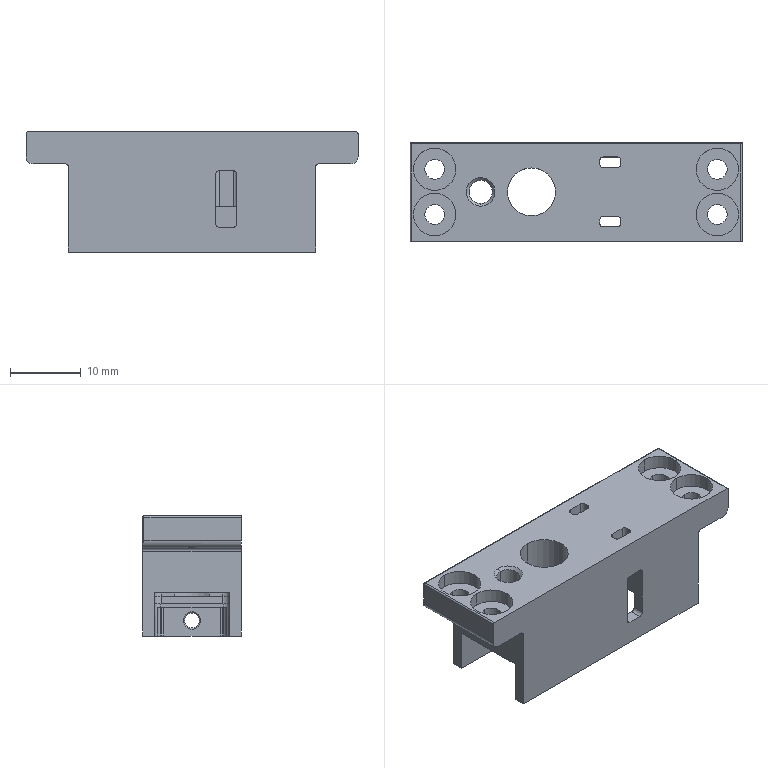NC program | NX | posted with a generic post | part box 47 x 14 x 17 mm
Lines 1055 to 1942 of 3166:
(CAVITY_MILL_COPY_COPY_COPY_COPY , TOOL : D1)
N2108 T22 M6
N2110 G54
N2112 G17 G0 G90 X-5.75 Y-1.208 B0. C0. S9200 M3
N2114 G43 Z30. H22
N2116 Z-0.065
N2118 G94 G3 X-5.85 Y-1.644 R1. F1000.
N2120 G1 Y-2.5 F850.
N2122 X-4.996
N2124 G3 X-4.696 Y-2.4 R0.5
N2126 G1 X-5.75 Y-1.208 Z-0.13 F8000.
N2128 G3 X-5.85 Y-1.644 R1. F1000.
N2130 G1 Y-2.5 F850.
N2132 X-4.996
N2134 G3 X-4.696 Y-2.4 R0.5
N2136 G1 X-5.75 Y-1.208 Z-0.195 F8000.
N2138 G3 X-5.85 Y-1.644 R1. F1000.
N2140 G1 Y-2.5 F850.
N2142 X-4.996
N2144 G3 X-4.696 Y-2.4 R0.5
N2146 G1 X-5.75 Y-1.208 Z-0.26 F8000.
N2148 G3 X-5.85 Y-1.644 R1. F1000.
N2150 G1 Y-2.5 F850.
N2152 X-4.996
N2154 G3 X-4.696 Y-2.4 R0.5
N2156 G1 X-5.75 Y-1.208 Z-0.325 F8000.
N2158 G3 X-5.85 Y-1.644 R1. F1000.
N2160 G1 Y-2.5 F850.
N2162 X-4.995
N2164 G3 X-4.695 Y-2.4 R0.5
N2166 G1 X-5.75 Y-1.208 Z-0.39 F8000.
N2168 G3 X-5.85 Y-1.644 R1. F1000.
N2170 G1 Y-2.5 F850.
N2172 X-4.995
N2174 G3 X-4.695 Y-2.4 R0.5
N2176 G1 X-5.75 Y-1.208 Z-0.455 F8000.
N2178 G3 X-5.85 Y-1.643 R1. F1000.
N2180 G1 Y-2.5 F850.
N2182 X-4.995
N2184 G3 X-4.695 Y-2.4 R0.5
N2186 G1 X-5.75 Y-1.207 Z-0.52 F8000.
N2188 G3 X-5.85 Y-1.643 R1. F1000.
N2190 G1 Y-2.5 F850.
N2192 X-4.995
N2194 G3 X-4.695 Y-2.4 R0.5
N2196 G1 X-5.75 Y-1.207 Z-0.585 F8000.
N2198 G3 X-5.85 Y-1.643 R1. F1000.
N2200 G1 Y-2.5 F850.
N2202 X-4.994
N2204 G3 X-4.694 Y-2.4 R0.5
N2206 G1 X-5.75 Y-1.207 Z-0.649 F8000.
N2208 G3 X-5.85 Y-1.643 R1. F1000.
N2210 G1 Y-2.5 F850.
N2212 X-4.994
N2214 G3 X-4.694 Y-2.4 R0.5
N2216 G1 X-5.75 Y-1.207 Z-0.714 F8000.
N2218 G3 X-5.85 Y-1.643 R1. F1000.
N2220 G1 Y-2.5 F850.
N2222 X-4.994
N2224 G3 X-4.694 Y-2.4 R0.5
N2226 G1 X-5.75 Y-1.207 Z-0.779 F8000.
N2228 G3 X-5.85 Y-1.643 R1. F1000.
N2230 G1 Y-2.5 F850.
N2232 X-4.994
N2234 G3 X-4.694 Y-2.4 R0.5
N2236 G1 X-5.75 Y-1.207 Z-0.844 F8000.
N2238 G3 X-5.85 Y-1.643 R1. F1000.
N2240 G1 Y-2.5 F850.
N2242 X-4.994
N2244 G3 X-4.694 Y-2.4 R0.5
N2246 G1 X-5.75 Y-1.207 Z-0.909 F8000.
N2248 G3 X-5.85 Y-1.643 R1. F1000.
N2250 G1 Y-2.5 F850.
N2252 X-4.993
N2254 G3 X-4.693 Y-2.4 R0.5
N2256 G1 X-5.75 Y-1.207 Z-0.974 F8000.
N2258 G3 X-5.85 Y-1.643 R1. F1000.
N2260 G1 Y-2.5 F850.
N2262 X-4.993
N2264 G3 X-4.693 Y-2.4 R0.5
N2266 G1 X-5.75 Y-1.207 Z-1.039 F8000.
N2268 G3 X-5.85 Y-1.643 R1. F1000.
N2270 G1 Y-2.5 F850.
N2272 X-4.993
N2274 G3 X-4.693 Y-2.4 R0.5
N2276 G1 X-5.75 Y-1.207 Z-1.104 F8000.
N2278 G3 X-5.85 Y-1.643 R1. F1000.
N2280 G1 Y-2.5 F850.
N2282 X-4.993
N2284 G3 X-4.693 Y-2.4 R0.5
N2286 G1 X-5.75 Y-1.207 Z-1.169 F8000.
N2288 G3 X-5.85 Y-1.643 R1. F1000.
N2290 G1 Y-2.5 F850.
N2292 X-4.992
N2294 G3 X-4.692 Y-2.4 R0.5
N2296 G1 X-5.75 Y-1.207 Z-1.234 F8000.
N2298 G3 X-5.85 Y-1.643 R1. F1000.
N2300 G1 Y-2.5 F850.
N2302 X-4.992
N2304 G3 X-4.692 Y-2.4 R0.5
N2306 G1 X-5.75 Y-1.207 Z-1.299 F8000.
N2308 G3 X-5.85 Y-1.643 R1. F1000.
N2310 G1 Y-2.5 F850.
N2312 X-4.992
N2314 G3 X-5.224 Y-2.4 R1.
N2316 G1 X-5.75 Y-1.207 Z-1.364 F8000.
N2318 G3 X-5.85 Y-1.642 R1. F1000.
N2320 G1 Y-2.5 F850.
N2322 X-4.992
N2324 G3 X-5.223 Y-2.4 R1.
N2326 G1 X-5.75 Y-1.206 Z-1.429 F8000.
N2328 G3 X-5.85 Y-1.642 R1. F1000.
N2330 G1 Y-2.5 F850.
N2332 X-4.991
N2334 G3 X-5.222 Y-2.4 R1.
N2336 G1 X-5.75 Y-1.206 Z-1.494 F8000.
N2338 G3 X-5.85 Y-1.642 R1. F1000.
N2340 G1 Y-2.5 F850.
N2342 X-4.991
N2344 G3 X-5.222 Y-2.4 R1.
N2346 G1 X-5.75 Y-1.206 Z-1.559 F8000.
N2348 G3 X-5.85 Y-1.642 R1. F1000.
N2350 G1 Y-2.5 F850.
N2352 X-4.991
N2354 G3 X-5.221 Y-2.4 R1.
N2356 G1 X-5.75 Y-1.206 Z-1.624 F8000.
N2358 G3 X-5.85 Y-1.642 R1. F1000.
N2360 G1 Y-2.5 F850.
N2362 X-4.99
N2364 G3 X-5.22 Y-2.4 R1.
N2366 G1 X-5.75 Y-1.206 Z-1.689 F8000.
N2368 G3 X-5.85 Y-1.642 R1. F1000.
N2370 G1 Y-2.5 F850.
N2372 X-4.99
N2374 G3 X-5.219 Y-2.4 R1.
N2376 G1 X-5.75 Y-1.206 Z-1.754 F8000.
N2378 G3 X-5.85 Y-1.642 R1. F1000.
N2380 G1 Y-2.5 F850.
N2382 X-4.99
N2384 G3 X-5.219 Y-2.4 R1.
N2386 G1 X-5.75 Y-1.206 Z-1.818 F8000.
N2388 G3 X-5.85 Y-1.642 R1. F1000.
N2390 G1 Y-2.5 F850.
N2392 X-4.99
N2394 G3 X-5.218 Y-2.4 R1.
N2396 G1 X-5.75 Y-1.206 Z-1.883 F8000.
N2398 G3 X-5.85 Y-1.642 R1. F1000.
N2400 G1 Y-2.5 F850.
N2402 X-4.989
N2404 G3 X-5.217 Y-2.4 R1.
N2406 G1 X-5.75 Y-1.206 Z-1.948 F8000.
N2408 G3 X-5.85 Y-1.642 R1. F1000.
N2410 G1 Y-2.5 F850.
N2412 X-4.989
N2414 G3 X-5.216 Y-2.4 R1.
N2416 G1 X-5.75 Y-1.206 Z-2.013 F8000.
N2418 G3 X-5.85 Y-1.642 R1. F1000.
N2420 G1 Y-2.5 F850.
N2422 X-4.989
N2424 G3 X-5.216 Y-2.4 R1.
N2426 G1 X-5.75 Y-1.206 Z-2.078 F8000.
N2428 G3 X-5.85 Y-1.642 R1. F1000.
N2430 G1 Y-2.5 F850.
N2432 X-4.989
N2434 G3 X-5.215 Y-2.4 R1.
N2436 G1 X-5.75 Y-1.206 Z-2.143 F8000.
N2438 G3 X-5.85 Y-1.642 R1. F1000.
N2440 G1 Y-2.5 F850.
N2442 X-4.988
N2444 G3 X-5.214 Y-2.4 R1.
N2446 G1 X-5.75 Y-1.206 Z-2.208 F8000.
N2448 G3 X-5.85 Y-1.641 R1. F1000.
N2450 G1 Y-2.5 F850.
N2452 X-4.988
N2454 G3 X-5.213 Y-2.4 R1.
N2456 G1 X-5.75 Y-1.205 Z-2.273 F8000.
N2458 G3 X-5.85 Y-1.641 R1. F1000.
N2460 G1 Y-2.5 F850.
N2462 X-4.988
N2464 G3 X-5.212 Y-2.4 R1.
N2466 G1 X-5.75 Y-1.205 Z-2.338 F8000.
N2468 G3 X-5.85 Y-1.641 R1. F1000.
N2470 G1 Y-2.5 F850.
N2472 X-4.987
N2474 G3 X-5.212 Y-2.4 R1.
N2476 G1 X-5.75 Y-1.205 Z-2.403 F8000.
N2478 G3 X-5.85 Y-1.641 R1. F1000.
N2480 G1 Y-2.5 F850.
N2482 X-4.987
N2484 G3 X-5.211 Y-2.4 R1.
N2486 G1 X-5.75 Y-1.205 Z-2.468 F8000.
N2488 G3 X-5.85 Y-1.641 R1. F1000.
N2490 G1 Y-2.5 F850.
N2492 X-4.987
N2494 G3 X-5.21 Y-2.4 R1.
N2496 G1 X-5.75 Y-1.205 Z-2.533 F8000.
N2498 G3 X-5.85 Y-1.641 R1. F1000.
N2500 G1 Y-2.5 F850.
N2502 X-4.986
N2504 G3 X-5.209 Y-2.4 R1.
N2506 G1 X-5.75 Y-1.205 Z-2.598 F8000.
N2508 G3 X-5.85 Y-1.641 R1. F1000.
N2510 G1 Y-2.5 F850.
N2512 X-4.986
N2514 G3 X-5.208 Y-2.4 R1.
N2516 G1 X-5.75 Y-1.205 Z-2.663 F8000.
N2518 G3 X-5.85 Y-1.641 R1. F1000.
N2520 G1 Y-2.5 F850.
N2522 X-4.986
N2524 G3 X-5.207 Y-2.4 R1.
N2526 G1 X-5.75 Y-1.205 Z-2.728 F8000.
N2528 G3 X-5.85 Y-1.641 R1. F1000.
N2530 G1 Y-2.5 F850.
N2532 X-4.985
N2534 G3 X-5.206 Y-2.4 R1.
N2536 G1 X-5.75 Y-1.205 Z-2.793 F8000.
N2538 G3 X-5.85 Y-1.641 R1. F1000.
N2540 G1 Y-2.5 F850.
N2542 X-4.985
N2544 G3 X-5.206 Y-2.4 R1.
N2546 G1 X-5.75 Y-1.205 Z-2.858 F8000.
N2548 G3 X-5.85 Y-1.641 R1. F1000.
N2550 G1 Y-2.5 F850.
N2552 X-4.985
N2554 G3 X-5.206 Y-2.4 R1.
N2556 G1 X-5.75 Y-1.205 Z-2.923 F8000.
N2558 G3 X-5.85 Y-1.641 R1. F1000.
N2560 G1 Y-2.5 F850.
N2562 X-4.985
N2564 G3 X-5.206 Y-2.4 R1.
N2566 G1 X-5.75 Y-1.205 Z-2.988 F8000.
N2568 G3 X-5.85 Y-1.64 R1. F1000.
N2570 G1 Y-2.5 F850.
N2572 X-4.985
N2574 G3 X-5.206 Y-2.4 R1.
N2576 G1 X-5.75 Y-1.204 Z-3.052 F8000.
N2578 G3 X-5.85 Y-1.64 R1. F1000.
N2580 G1 Y-2.5 F850.
N2582 X-4.985
N2584 G3 X-5.206 Y-2.4 R1.
N2586 G1 X-5.75 Y-1.204 Z-3.117 F8000.
N2588 G3 X-5.85 Y-1.64 R1. F1000.
N2590 G1 Y-2.5 F850.
N2592 X-4.985
N2594 G3 X-5.206 Y-2.4 R1.
N2596 G1 X-5.75 Y-1.204 Z-3.182 F8000.
N2598 G3 X-5.85 Y-1.64 R1. F1000.
N2600 G1 Y-2.5 F850.
N2602 X-4.985
N2604 G3 X-5.206 Y-2.4 R1.
N2606 G1 X-5.75 Y-1.204 Z-3.247 F8000.
N2608 G3 X-5.85 Y-1.64 R1. F1000.
N2610 G1 Y-2.5 F850.
N2612 X-4.985
N2614 G3 X-5.206 Y-2.4 R1.
N2616 G1 X-5.75 Y-1.204 Z-3.312 F8000.
N2618 G3 X-5.85 Y-1.64 R1. F1000.
N2620 G1 Y-2.5 F850.
N2622 X-4.985
N2624 G3 X-5.206 Y-2.4 R1.
N2626 G1 X-5.75 Y-1.204 Z-3.377 F8000.
N2628 G3 X-5.85 Y-1.64 R1. F1000.
N2630 G1 Y-2.5 F850.
N2632 X-4.985
N2634 G3 X-5.206 Y-2.4 R1.
N2636 G1 X-5.75 Y-1.204 Z-3.442 F8000.
N2638 G3 X-5.85 Y-1.64 R1. F1000.
N2640 G1 Y-2.5 F850.
N2642 X-4.985
N2644 G3 X-5.206 Y-2.4 R1.
N2646 G1 X-5.75 Y-1.204 Z-3.507 F8000.
N2648 G3 X-5.85 Y-1.64 R1. F1000.
N2650 G1 Y-2.5 F850.
N2652 X-4.985
N2654 G3 X-5.206 Y-2.4 R1.
N2656 G1 X-5.75 Y-1.204 Z-3.572 F8000.
N2658 G3 X-5.85 Y-1.64 R1. F1000.
N2660 G1 Y-2.5 F850.
N2662 X-4.985
N2664 G3 X-5.206 Y-2.4 R1.
N2666 G1 X-5.75 Y-1.204 Z-3.637 F8000.
N2668 G3 X-5.85 Y-1.64 R1. F1000.
N2670 G1 Y-2.5 F850.
N2672 X-4.985
N2674 G3 X-5.206 Y-2.4 R1.
N2676 G1 X-5.75 Y-1.204 Z-3.702 F8000.
N2678 G3 X-5.85 Y-1.64 R1. F1000.
N2680 G1 Y-2.5 F850.
N2682 X-4.985
N2684 G3 X-5.206 Y-2.4 R1.
N2686 G1 X-5.75 Y-1.204 Z-3.767 F8000.
N2688 G3 X-5.85 Y-1.64 R1. F1000.
N2690 G1 Y-2.5 F850.
N2692 X-4.985
N2694 G3 X-5.205 Y-2.4 R1.
N2696 G1 X-5.75 Y-1.204 Z-3.832 F8000.
N2698 G3 X-5.85 Y-1.64 R1. F1000.
N2700 G1 Y-2.5 F850.
N2702 X-4.985
N2704 G3 X-5.205 Y-2.4 R1.
N2706 G1 X-5.75 Y-1.204 Z-3.897 F8000.
N2708 G3 X-5.85 Y-1.64 R1. F1000.
N2710 G1 Y-2.5 F850.
N2712 X-4.985
N2714 G3 X-5.205 Y-2.4 R1.
N2716 G1 X-5.75 Y-1.204 Z-3.962 F8000.
N2718 G3 X-5.85 Y-1.64 R1. F1000.
N2720 G1 Y-2.5 F850.
N2722 X-4.985
N2724 G3 X-5.205 Y-2.4 R1.
N2726 G1 X-5.75 Y-1.204 Z-4.027 F8000.
N2728 G3 X-5.85 Y-1.64 R1. F1000.
N2730 G1 Y-2.5 F850.
N2732 X-4.985
N2734 G3 X-5.205 Y-2.4 R1.
N2736 G1 X-5.75 Y-1.204 Z-4.092 F8000.
N2738 G3 X-5.85 Y-1.64 R1. F1000.
N2740 G1 Y-2.5 F850.
N2742 X-4.985
N2744 G3 X-5.205 Y-2.4 R1.
N2746 G1 X-5.75 Y-1.204 Z-4.157 F8000.
N2748 G3 X-5.85 Y-1.64 R1. F1000.
N2750 G1 Y-2.5 F850.
N2752 X-4.985
N2754 G3 X-5.205 Y-2.4 R1.
N2756 G1 X-5.75 Y-1.204 Z-4.221 F8000.
N2758 G3 X-5.85 Y-1.64 R1. F1000.
N2760 G1 Y-2.5 F850.
N2762 X-4.985
N2764 G3 X-5.205 Y-2.4 R1.
N2766 G1 X-5.75 Y-1.204 Z-4.286 F8000.
N2768 G3 X-5.85 Y-1.64 R1. F1000.
N2770 G1 Y-2.5 F850.
N2772 X-4.985
N2774 G3 X-5.205 Y-2.4 R1.
N2776 G1 X-5.75 Y-1.204 Z-4.351 F8000.
N2778 G3 X-5.85 Y-1.64 R1. F1000.
N2780 G1 Y-2.5 F850.
N2782 X-4.985
N2784 G3 X-5.205 Y-2.4 R1.
N2786 G1 X-5.75 Y-1.204 Z-4.416 F8000.
N2788 G3 X-5.85 Y-1.64 R1. F1000.
N2790 G1 Y-2.5 F850.
N2792 X-4.985
N2794 G3 X-5.205 Y-2.4 R1.
N2796 G1 X-5.75 Y-1.204 Z-4.481 F8000.
N2798 G3 X-5.85 Y-1.64 R1. F1000.
N2800 G1 Y-2.5 F850.
N2802 X-4.985
N2804 G3 X-5.203 Y-2.4 R1.
N2806 G1 X-5.75 Y-1.204 Z-4.546 F8000.
N2808 G3 X-5.85 Y-1.64 R1. F1000.
N2810 G1 Y-2.5 F850.
N2812 X-4.985
N2814 G3 X-5.205 Y-2.4 R1.
N2816 G1 X-5.75 Y-1.204 Z-4.611 F8000.
N2818 G3 X-5.85 Y-1.64 R1. F1000.
N2820 G1 Y-2.5 F850.
N2822 X-4.985
N2824 G3 X-5.205 Y-2.4 R1.
N2826 G1 X-5.75 Y-1.204 Z-4.676 F8000.
N2828 G3 X-5.85 Y-1.64 R1. F1000.
N2830 G1 Y-2.5 F850.
N2832 X-4.985
N2834 G3 X-5.205 Y-2.4 R1.
N2836 G1 X-5.75 Y-1.204 Z-4.741 F8000.
N2838 G3 X-5.85 Y-1.64 R1. F1000.
N2840 G1 Y-2.5 F850.
N2842 X-4.985
N2844 G3 X-5.205 Y-2.4 R1.
N2846 G1 X-5.75 Y-1.204 Z-4.806 F8000.
N2848 G3 X-5.85 Y-1.64 R1. F1000.
N2850 G1 Y-2.5 F850.
N2852 X-4.985
N2854 G3 X-5.205 Y-2.4 R1.
N2856 G1 X-5.75 Y-1.204 Z-4.871 F8000.
N2858 G3 X-5.85 Y-1.64 R1. F1000.
N2860 G1 Y-2.5 F850.
N2862 X-4.985
N2864 G3 X-5.205 Y-2.4 R1.
N2866 G1 X-5.75 Y-1.204 Z-4.936 F8000.
N2868 G3 X-5.85 Y-1.64 R1. F1000.
N2870 G1 Y-2.5 F850.
N2872 X-4.985
N2874 G3 X-5.205 Y-2.4 R1.
N2876 G1 X-5.75 Y-1.204 Z-5.001 F8000.
N2878 G3 X-5.85 Y-1.64 R1. F1000.
N2880 G1 Y-2.5 F850.
N2882 X-4.985
N2884 G3 X-5.205 Y-2.4 R1.
N2886 G1 X-5.75 Y-1.204 Z-5.066 F8000.
N2888 G3 X-5.85 Y-1.64 R1. F1000.
N2890 G1 Y-2.5 F850.
N2892 X-4.985
N2894 G3 X-5.205 Y-2.4 R1.
N2896 G1 X-5.75 Y-1.204 Z-5.131 F8000.
N2898 G3 X-5.85 Y-1.64 R1. F1000.
N2900 G1 Y-2.5 F850.
N2902 X-4.985
N2904 G3 X-5.205 Y-2.4 R1.
N2906 G1 X-5.75 Y-1.204 Z-5.196 F8000.
N2908 G3 X-5.85 Y-1.64 R1. F1000.
N2910 G1 Y-2.5 F850.
N2912 X-4.985
N2914 G3 X-5.205 Y-2.4 R1.
N2916 G1 X-5.75 Y-1.204 Z-5.261 F8000.
N2918 G3 X-5.85 Y-1.64 R1. F1000.
N2920 G1 Y-2.5 F850.
N2922 X-4.985
N2924 G3 X-5.205 Y-2.4 R1.
N2926 G1 X-5.75 Y-1.204 Z-5.326 F8000.
N2928 G3 X-5.85 Y-1.64 R1. F1000.
N2930 G1 Y-2.5 F850.
N2932 X-4.985
N2934 G3 X-5.205 Y-2.4 R1.
N2936 G1 X-5.75 Y-1.204 Z-5.39 F8000.
N2938 G3 X-5.85 Y-1.64 R1. F1000.
N2940 G1 Y-2.5 F850.
N2942 X-4.985
N2944 G3 X-5.205 Y-2.4 R1.
N2946 G1 X-5.75 Y-1.204 Z-5.455 F8000.
N2948 G3 X-5.85 Y-1.64 R1. F1000.
N2950 G1 Y-2.5 F850.
N2952 X-4.985
N2954 G3 X-5.205 Y-2.4 R1.
N2956 G1 X-5.75 Y-1.204 Z-5.52 F8000.
N2958 G3 X-5.85 Y-1.64 R1. F1000.
N2960 G1 Y-2.5 F850.
N2962 X-4.985
N2964 G3 X-5.205 Y-2.4 R1.
N2966 G1 X-5.75 Y-1.204 Z-5.585 F8000.
N2968 G3 X-5.85 Y-1.64 R1. F1000.
N2970 G1 Y-2.5 F850.
N2972 X-4.985
N2974 G3 X-5.205 Y-2.4 R1.
N2976 G1 X-5.75 Y-1.204 Z-5.65 F8000.
N2978 G3 X-5.85 Y-1.64 R1. F1000.
N2980 G1 Y-2.5 F850.
N2982 X-4.985
N2984 G3 X-5.205 Y-2.4 R1.
N2986 G1 X-5.75 Y-1.204 Z-5.715 F8000.
N2988 G3 X-5.85 Y-1.64 R1. F1000.
N2990 G1 Y-2.5 F850.
N2992 X-4.985
N2994 G3 X-5.205 Y-2.4 R1.
N2996 G1 X-5.75 Y-1.204 Z-5.78 F8000.
N2998 G3 X-5.85 Y-1.64 R1. F1000.
N3000 G1 Y-2.5 F850.
N3002 X-4.985
N3004 G3 X-5.205 Y-2.4 R1.
N3006 G1 X-5.75 Y-1.204 Z-5.845 F8000.
N3008 G3 X-5.85 Y-1.64 R1. F1000.
N3010 G1 Y-2.5 F850.
N3012 X-4.985
N3014 G3 X-5.205 Y-2.4 R1.
N3016 G1 X-5.75 Y-1.204 Z-5.91 F8000.
N3018 G3 X-5.85 Y-1.64 R1. F1000.
N3020 G1 Y-2.5 F850.
N3022 X-4.985
N3024 G3 X-5.205 Y-2.4 R1.
N3026 G1 X-5.75 Y-1.204 Z-5.975 F8000.
N3028 G3 X-5.85 Y-1.64 R1. F1000.
N3030 G1 Y-2.5 F850.
N3032 X-4.985
N3034 G3 X-5.205 Y-2.4 R1.
N3036 G1 X-5.75 Y-1.204 Z-6.04 F8000.
N3038 G3 X-5.85 Y-1.64 R1. F1000.
N3040 G1 Y-2.5 F850.
N3042 X-4.985
N3044 G3 X-5.205 Y-2.4 R1.
N3046 G1 X-5.75 Y-1.204 Z-6.105 F8000.
N3048 G3 X-5.85 Y-1.64 R1. F1000.
N3050 G1 Y-2.5 F850.
N3052 X-4.985
N3054 G3 X-5.205 Y-2.4 R1.
N3056 G1 X-5.75 Y-1.204 Z-6.17 F8000.
N3058 G3 X-5.85 Y-1.64 R1. F1000.
N3060 G1 Y-2.5 F850.
N3062 X-4.985
N3064 G3 X-5.205 Y-2.4 R1.
N3066 G1 X-5.75 Y-1.204 Z-6.235 F8000.
N3068 G3 X-5.85 Y-1.64 R1. F1000.
N3070 G1 Y-2.5 F850.
N3072 X-4.985
N3074 G3 X-5.205 Y-2.4 R1.
N3076 G1 X-5.75 Y-1.204 Z-6.3 F8000.
N3078 G3 X-5.85 Y-1.64 R1. F1000.
N3080 G1 Y-2.5 F850.
N3082 X-4.985
N3084 G3 X-5.205 Y-2.4 R1.
N3086 G1 X-5.75 Y-1.204 Z-6.365 F8000.
N3088 G3 X-5.85 Y-1.64 R1. F1000.
N3090 G1 Y-2.5 F850.
N3092 X-4.985
N3094 G3 X-5.205 Y-2.4 R1.
N3096 G1 X-5.75 Y-1.204 Z-6.43 F8000.
N3098 G3 X-5.85 Y-1.64 R1. F1000.
N3100 G1 Y-2.5 F850.
N3102 X-4.985
N3104 G3 X-5.205 Y-2.4 R1.
N3106 G1 X-5.75 Y-1.204 Z-6.495 F8000.
N3108 G3 X-5.85 Y-1.64 R1. F1000.
N3110 G1 Y-2.5 F850.
N3112 X-4.985
N3114 G3 X-5.205 Y-2.4 R1.
N3116 G1 X-5.75 Y-1.204 Z-6.56 F8000.
N3118 G3 X-5.85 Y-1.64 R1. F1000.
N3120 G1 Y-2.5 F850.
N3122 X-4.985
N3124 G3 X-5.205 Y-2.4 R1.
N3126 G1 X-5.75 Y-1.204 Z-6.624 F8000.
N3128 G3 X-5.85 Y-1.64 R1. F1000.
N3130 G1 Y-2.5 F850.
N3132 X-4.985
N3134 G3 X-5.205 Y-2.4 R1.
N3136 G1 X-5.75 Y-1.204 Z-6.689 F8000.
N3138 G3 X-5.85 Y-1.64 R1. F1000.
N3140 G1 Y-2.5 F850.
N3142 X-4.985
N3144 G3 X-5.205 Y-2.4 R1.
N3146 G1 X-5.75 Y-1.204 Z-6.754 F8000.
N3148 G3 X-5.85 Y-1.64 R1. F1000.
N3150 G1 Y-2.5 F850.
N3152 X-4.985
N3154 G3 X-5.205 Y-2.4 R1.
N3156 G1 X-5.75 Y-1.204 Z-6.819 F8000.
N3158 G3 X-5.85 Y-1.64 R1. F1000.
N3160 G1 Y-2.5 F850.
N3162 X-4.985
N3164 G3 X-5.205 Y-2.4 R1.
N3166 G1 X-5.75 Y-1.204 Z-6.884 F8000.
N3168 G3 X-5.85 Y-1.64 R1. F1000.
N3170 G1 Y-2.5 F850.
N3172 X-4.985
N3174 G3 X-5.205 Y-2.4 R1.
N3176 G1 X-5.75 Y-1.204 Z-6.949 F8000.
N3178 G3 X-5.85 Y-1.64 R1. F1000.
N3180 G1 Y-2.5 F850.
N3182 X-4.985
N3184 G3 X-5.205 Y-2.4 R1.
N3186 G1 X-5.75 Y-1.204 Z-7.014 F8000.
N3188 G3 X-5.85 Y-1.64 R1. F1000.
N3190 G1 Y-2.5 F850.
N3192 X-4.985
N3194 G3 X-5.205 Y-2.4 R1.
N3196 G1 X-5.75 Y-1.204 Z-7.079 F8000.
N3198 G3 X-5.85 Y-1.64 R1. F1000.
N3200 G1 Y-2.5 F850.
N3202 X-4.985
N3204 G3 X-5.205 Y-2.4 R1.
N3206 G1 X-5.75 Y-1.204 Z-7.144 F8000.
N3208 G3 X-5.85 Y-1.64 R1. F1000.
N3210 G1 Y-2.5 F850.
N3212 X-4.985
N3214 G3 X-5.205 Y-2.4 R1.
N3216 G1 X-5.75 Y-1.204 Z-7.209 F8000.
N3218 G3 X-5.85 Y-1.64 R1. F1000.
N3220 G1 Y-2.5 F850.
N3222 X-4.985
N3224 G3 X-5.205 Y-2.4 R1.
N3226 G1 X-5.75 Y-1.204 Z-7.274 F8000.
N3228 G3 X-5.85 Y-1.64 R1. F1000.
N3230 G1 Y-2.5 F850.
N3232 X-4.985
N3234 G3 X-5.205 Y-2.4 R1.
N3236 G1 X-5.75 Y-1.204 Z-7.339 F8000.
N3238 G3 X-5.85 Y-1.64 R1. F1000.
N3240 G1 Y-2.5 F850.
N3242 X-4.985
N3244 G3 X-5.205 Y-2.4 R1.
N3246 G1 X-5.75 Y-1.204 Z-7.404 F8000.
N3248 G3 X-5.85 Y-1.64 R1. F1000.
N3250 G1 Y-2.5 F850.
N3252 X-4.985
N3254 G3 X-5.205 Y-2.4 R1.
N3256 G1 X-5.75 Y-1.204 Z-7.469 F8000.
N3258 G3 X-5.85 Y-1.64 R1. F1000.
N3260 G1 Y-2.5 F850.
N3262 X-4.985
N3264 G3 X-5.205 Y-2.4 R1.
N3266 G1 X-5.75 Y-1.204 Z-7.534 F8000.
N3268 G3 X-5.85 Y-1.64 R1. F1000.
N3270 G1 Y-2.5 F850.
N3272 X-4.985
N3274 G3 X-5.205 Y-2.4 R1.
N3276 G1 X-5.75 Y-1.204 Z-7.599 F8000.
N3278 G3 X-5.85 Y-1.64 R1. F1000.
N3280 G1 Y-2.5 F850.
N3282 X-4.985
N3284 G3 X-5.205 Y-2.4 R1.
N3286 G1 X-5.75 Y-1.204 Z-7.664 F8000.
N3288 G3 X-5.85 Y-1.64 R1. F1000.
N3290 G1 Y-2.5 F850.
N3292 X-4.985
N3294 G3 X-5.205 Y-2.4 R1.
N3296 G1 X-5.75 Y-1.204 Z-7.729 F8000.
N3298 G3 X-5.85 Y-1.64 R1. F1000.
N3300 G1 Y-2.5 F850.
N3302 X-4.985
N3304 G3 X-5.205 Y-2.4 R1.
N3306 G1 X-5.75 Y-1.204 Z-7.793 F8000.
N3308 G3 X-5.85 Y-1.64 R1. F1000.
N3310 G1 Y-2.5 F850.
N3312 X-4.985
N3314 G3 X-5.205 Y-2.4 R1.
N3316 G1 X-5.75 Y-1.204 Z-7.858 F8000.
N3318 G3 X-5.85 Y-1.64 R1. F1000.
N3320 G1 Y-2.5 F850.
N3322 X-4.985
N3324 G3 X-5.205 Y-2.4 R1.
N3326 G1 X-5.75 Y-1.204 Z-7.923 F8000.
N3328 G3 X-5.85 Y-1.64 R1. F1000.
N3330 G1 Y-2.5 F850.
N3332 X-4.985
N3334 G3 X-5.205 Y-2.4 R1.
N3336 G1 X-5.75 Y-1.204 Z-7.988 F8000.
N3338 G3 X-5.85 Y-1.64 R1. F1000.
N3340 G1 Y-2.5 F850.
N3342 X-4.985
N3344 G3 X-5.205 Y-2.4 R1.
N3346 G1 X-5.75 Y-1.204 Z-8.053 F8000.
N3348 G3 X-5.85 Y-1.64 R1. F1000.
N3350 G1 Y-2.5 F850.
N3352 X-4.985
N3354 G3 X-5.205 Y-2.4 R1.
N3356 G1 X-5.75 Y-1.204 Z-8.118 F8000.
N3358 G3 X-5.85 Y-1.64 R1. F1000.
N3360 G1 Y-2.5 F850.
N3362 X-4.985
N3364 G3 X-5.205 Y-2.4 R1.
N3366 G1 X-5.75 Y-1.204 Z-8.183 F8000.
N3368 G3 X-5.85 Y-1.64 R1. F1000.
N3370 G1 Y-2.5 F850.
N3372 X-4.985
N3374 G3 X-5.205 Y-2.4 R1.
N3376 G1 X-5.75 Y-1.204 Z-8.248 F8000.
N3378 G3 X-5.85 Y-1.64 R1. F1000.
N3380 G1 Y-2.5 F850.
N3382 X-4.985
N3384 G3 X-5.204 Y-2.4 R1.
N3386 G1 X-5.75 Y-1.204 Z-8.313 F8000.
N3388 G3 X-5.85 Y-1.64 R1. F1000.
N3390 G1 Y-2.5 F850.
N3392 X-4.985
N3394 G3 X-5.205 Y-2.4 R1.
N3396 G1 X-5.75 Y-1.204 Z-8.378 F8000.
N3398 G3 X-5.85 Y-1.64 R1. F1000.
N3400 G1 Y-2.5 F850.
N3402 X-4.985
N3404 G3 X-5.205 Y-2.4 R1.
N3406 G1 X-5.75 Y-1.204 Z-8.443 F8000.
N3408 G3 X-5.85 Y-1.64 R1. F1000.
N3410 G1 Y-2.5 F850.
N3412 X-4.985
N3414 G3 X-5.205 Y-2.4 R1.
N3416 G1 X-5.75 Y-1.204 Z-8.508 F8000.
N3418 G3 X-5.85 Y-1.64 R1. F1000.
N3420 G1 Y-2.5 F850.
N3422 X-4.985
N3424 G3 X-5.205 Y-2.4 R1.
N3426 G1 X-5.75 Y-1.204 Z-8.573 F8000.
N3428 G3 X-5.85 Y-1.64 R1. F1000.
N3430 G1 Y-2.5 F850.
N3432 X-4.985
N3434 G3 X-5.205 Y-2.4 R1.
N3436 G1 X-5.75 Y-1.204 Z-8.638 F8000.
N3438 G3 X-5.85 Y-1.64 R1. F1000.
N3440 G1 Y-2.5 F850.
N3442 X-4.985
N3444 G3 X-5.205 Y-2.4 R1.
N3446 G1 X-5.75 Y-1.204 Z-8.703 F8000.
N3448 G3 X-5.85 Y-1.64 R1. F1000.
N3450 G1 Y-2.5 F850.
N3452 X-4.985
N3454 G3 X-5.205 Y-2.4 R1.
N3456 G1 X-5.75 Y-1.204 Z-8.768 F8000.
N3458 G3 X-5.85 Y-1.64 R1. F1000.
N3460 G1 Y-2.5 F850.
N3462 X-4.985
N3464 G3 X-5.205 Y-2.4 R1.
N3466 G1 X-5.75 Y-1.204 Z-8.833 F8000.
N3468 G3 X-5.85 Y-1.64 R1. F1000.
N3470 G1 Y-2.5 F850.
N3472 X-4.985
N3474 G3 X-5.205 Y-2.4 R1.
N3476 G1 X-5.75 Y-1.204 Z-8.898 F8000.
N3478 G3 X-5.85 Y-1.64 R1. F1000.
N3480 G1 Y-2.5 F850.
N3482 X-4.985
N3484 G3 X-5.205 Y-2.4 R1.
N3486 G1 X-5.75 Y-1.204 Z-8.963 F8000.
N3488 G3 X-5.85 Y-1.64 R1. F1000.
N3490 G1 Y-2.5 F850.
N3492 X-4.985
N3494 G3 X-5.205 Y-2.4 R1.
N3496 G1 X-5.75 Y-1.204 Z-9.027 F8000.
N3498 G3 X-5.85 Y-1.64 R1. F1000.
N3500 G1 Y-2.5 F850.
N3502 X-4.985
N3504 G3 X-5.205 Y-2.4 R1.
N3506 G1 X-5.75 Y-1.204 Z-9.092 F8000.
N3508 G3 X-5.85 Y-1.64 R1. F1000.
N3510 G1 Y-2.5 F850.
N3512 X-4.985
N3514 G3 X-5.205 Y-2.4 R1.
N3516 G1 X-5.75 Y-1.204 Z-9.157 F8000.
N3518 G3 X-5.85 Y-1.64 R1. F1000.
N3520 G1 Y-2.5 F850.
N3522 X-4.985
N3524 G3 X-5.205 Y-2.4 R1.
N3526 G1 X-5.75 Y-1.204 Z-9.222 F8000.
N3528 G3 X-5.85 Y-1.64 R1. F1000.
N3530 G1 Y-2.5 F850.
N3532 X-4.985
N3534 G3 X-5.205 Y-2.4 R1.
N3536 G1 X-5.75 Y-1.204 Z-9.287 F8000.
N3538 G3 X-5.85 Y-1.64 R1. F1000.
N3540 G1 Y-2.5 F850.
N3542 X-4.985
N3544 G3 X-5.205 Y-2.4 R1.
N3546 G1 X-5.75 Y-1.204 Z-9.352 F8000.
N3548 G3 X-5.85 Y-1.64 R1. F1000.
N3550 G1 Y-2.5 F850.
N3552 X-4.985
N3554 G3 X-5.205 Y-2.4 R1.
N3556 G1 X-5.75 Y-1.204 Z-9.417 F8000.
N3558 G3 X-5.85 Y-1.64 R1. F1000.
N3560 G1 Y-2.5 F850.
N3562 X-4.985
N3564 G3 X-5.205 Y-2.4 R1.
N3566 G1 X-5.75 Y-1.204 Z-9.482 F8000.
N3568 G3 X-5.85 Y-1.64 R1. F1000.
N3570 G1 Y-2.5 F850.
N3572 X-4.985
N3574 G3 X-5.205 Y-2.4 R1.
N3576 G1 X-5.75 Y-1.204 Z-9.547 F8000.
N3578 G3 X-5.85 Y-1.64 R1. F1000.
N3580 G1 Y-2.5 F850.
N3582 X-4.985
N3584 G3 X-5.205 Y-2.4 R1.
N3586 G1 X-5.75 Y-1.204 Z-9.612 F8000.
N3588 G3 X-5.85 Y-1.64 R1. F1000.
N3590 G1 Y-2.5 F850.
N3592 X-4.985
N3594 G3 X-5.204 Y-2.4 R1.
N3596 G1 X-5.75 Y-1.204 Z-9.677 F8000.
N3598 G3 X-5.85 Y-1.64 R1. F1000.
N3600 G1 Y-2.5 F850.
N3602 X-4.985
N3604 G3 X-5.204 Y-2.4 R1.
N3606 G1 X-5.75 Y-1.204 Z-9.742 F8000.
N3608 G3 X-5.85 Y-1.64 R1. F1000.
N3610 G1 Y-2.5 F850.
N3612 X-4.985
N3614 G3 X-5.204 Y-2.4 R1.
N3616 G1 X-5.75 Y-1.204 Z-9.807 F8000.
N3618 G3 X-5.85 Y-1.64 R1. F1000.
N3620 G1 Y-2.5 F850.
N3622 X-4.985
N3624 G3 X-5.204 Y-2.4 R1.
N3626 G1 X-5.75 Y-1.204 Z-9.872 F8000.
N3628 G3 X-5.85 Y-1.64 R1. F1000.
N3630 G1 Y-2.5 F850.
N3632 X-4.985
N3634 G3 X-5.204 Y-2.4 R1.
N3636 G1 X-5.75 Y-1.204 Z-9.937 F8000.
N3638 G3 X-5.85 Y-1.64 R1. F1000.
N3640 G1 Y-2.5 F850.
N3642 X-4.985
N3644 G3 X-5.204 Y-2.4 R1.
N3646 G1 X-5.75 Y-1.204 Z-10.002 F8000.
N3648 G3 X-5.85 Y-1.64 R1. F1000.
N3650 G1 Y-2.5 F850.
N3652 X-4.985
N3654 G3 X-5.204 Y-2.4 R1.
N3656 G1 X-5.75 Y-1.204 Z-10.067 F8000.
N3658 G3 X-5.85 Y-1.64 R1. F1000.
N3660 G1 Y-2.5 F850.
N3662 X-4.985
N3664 G3 X-5.204 Y-2.4 R1.
N3666 G1 X-5.75 Y-1.204 Z-10.132 F8000.
N3668 G3 X-5.85 Y-1.64 R1. F1000.
N3670 G1 Y-2.5 F850.
N3672 X-4.985
N3674 G3 X-5.204 Y-2.4 R1.
N3676 G1 X-5.75 Y-1.204 Z-10.196 F8000.
N3678 G3 X-5.85 Y-1.64 R1. F1000.
N3680 G1 Y-2.5 F850.
N3682 X-4.985
N3684 G3 X-5.204 Y-2.4 R1.
N3686 G1 X-5.75 Y-1.204 Z-10.261 F8000.
N3688 G3 X-5.85 Y-1.64 R1. F1000.
N3690 G1 Y-2.5 F850.
N3692 X-4.985
N3694 G3 X-5.204 Y-2.4 R1.
N3696 G1 X-5.75 Y-1.204 Z-10.326 F8000.
N3698 G3 X-5.85 Y-1.64 R1. F1000.
N3700 G1 Y-2.5 F850.
N3702 X-4.985
N3704 G3 X-5.204 Y-2.4 R1.
N3706 G1 X-5.75 Y-1.204 Z-10.391 F8000.
N3708 G3 X-5.85 Y-1.64 R1. F1000.
N3710 G1 Y-2.5 F850.
N3712 X-4.985
N3714 G3 X-5.204 Y-2.4 R1.
N3716 G1 X-5.75 Y-1.204 Z-10.456 F8000.
N3718 G3 X-5.85 Y-1.64 R1. F1000.
N3720 G1 Y-2.5 F850.
N3722 X-4.985
N3724 G3 X-5.204 Y-2.4 R1.
N3726 G1 X-5.75 Y-1.204 Z-10.521 F8000.
N3728 G3 X-5.85 Y-1.64 R1. F1000.
N3730 G1 Y-2.5 F850.
N3732 X-4.985
N3734 G3 X-5.204 Y-2.4 R1.
N3736 G1 X-5.75 Y-1.204 Z-10.586 F8000.
N3738 G3 X-5.85 Y-1.64 R1. F1000.
N3740 G1 Y-2.5 F850.
N3742 X-4.985
N3744 G3 X-5.204 Y-2.4 R1.
N3746 G1 X-5.75 Y-1.204 Z-10.651 F8000.
N3748 G3 X-5.85 Y-1.64 R1. F1000.
N3750 G1 Y-2.5 F850.
N3752 X-4.985
N3754 G3 X-5.204 Y-2.4 R1.
N3756 G1 X-5.75 Y-1.204 Z-10.716 F8000.
N3758 G3 X-5.85 Y-1.64 R1. F1000.
N3760 G1 Y-2.5 F850.
N3762 X-4.985
N3764 G3 X-5.204 Y-2.4 R1.
N3766 G1 X-5.75 Y-1.204 Z-10.781 F8000.
N3768 G3 X-5.85 Y-1.64 R1. F1000.
N3770 G1 Y-2.5 F850.
N3772 X-4.985
N3774 G3 X-5.204 Y-2.4 R1.
N3776 G1 X-5.75 Y-1.204 Z-10.846 F8000.
N3778 G3 X-5.85 Y-1.64 R1. F1000.
N3780 G1 Y-2.5 F850.
N3782 X-4.985
N3784 G3 X-5.204 Y-2.4 R1.
N3786 G1 X-5.75 Y-1.204 Z-10.911 F8000.
N3788 G3 X-5.85 Y-1.64 R1. F1000.
N3790 G1 Y-2.5 F850.
N3792 X-4.985
N3794 G3 X-5.204 Y-2.4 R1.
N3796 G1 X-5.75 Y-1.204 Z-10.976 F8000.
N3798 G3 X-5.85 Y-1.64 R1. F1000.
N3800 G1 Y-2.5 F850.
N3802 X-4.985
N3804 G3 X-5.204 Y-2.4 R1.
N3806 G1 X-5.75 Y-1.204 Z-11.041 F8000.
N3808 G3 X-5.85 Y-1.64 R1. F1000.
N3810 G1 Y-2.5 F850.
N3812 X-4.985
N3814 G3 X-5.204 Y-2.4 R1.
N3816 G1 X-5.75 Y-1.204 Z-11.106 F8000.
N3818 G3 X-5.85 Y-1.64 R1. F1000.
N3820 G1 Y-2.5 F850.
N3822 X-4.982
N3824 G3 X-5.197 Y-2.4 R1.
N3826 G1 X-5.75 Y-1.204 Z-11.171 F8000.
N3828 G3 X-5.85 Y-1.64 R1. F1000.
N3830 G1 Y-2.5 F850.
N3832 X-4.982
N3834 G3 X-5.197 Y-2.4 R1.
N3836 G1 X-5.75 Y-1.204 Z-11.236 F8000.
N3838 G3 X-5.85 Y-1.64 R1. F1000.
N3840 G1 Y-2.5 F850.
N3842 X-4.982
N3844 G3 X-5.197 Y-2.4 R1.
N3846 G1 X-5.75 Y-1.204 Z-11.301 F8000.
N3848 G3 X-5.85 Y-1.64 R1. F1000.
N3850 G1 Y-2.5 F850.
N3852 X-4.982
N3854 G3 X-5.197 Y-2.4 R1.
N3856 G1 X-5.75 Y-1.204 Z-11.365 F8000.
N3858 G3 X-5.85 Y-1.64 R1. F1000.
N3860 G1 Y-2.5 F850.
N3862 X-4.982
N3864 G3 X-5.197 Y-2.4 R1.
N3866 G1 X-5.75 Y-1.204 Z-11.43 F8000.
N3868 G3 X-5.85 Y-1.64 R1. F1000.
N3870 G1 Y-2.5 F850.
N3872 X-4.982
N3874 G3 X-5.197 Y-2.4 R1.
N3876 G1 X-5.748 Y-1.202 Z-11.495 F8000.